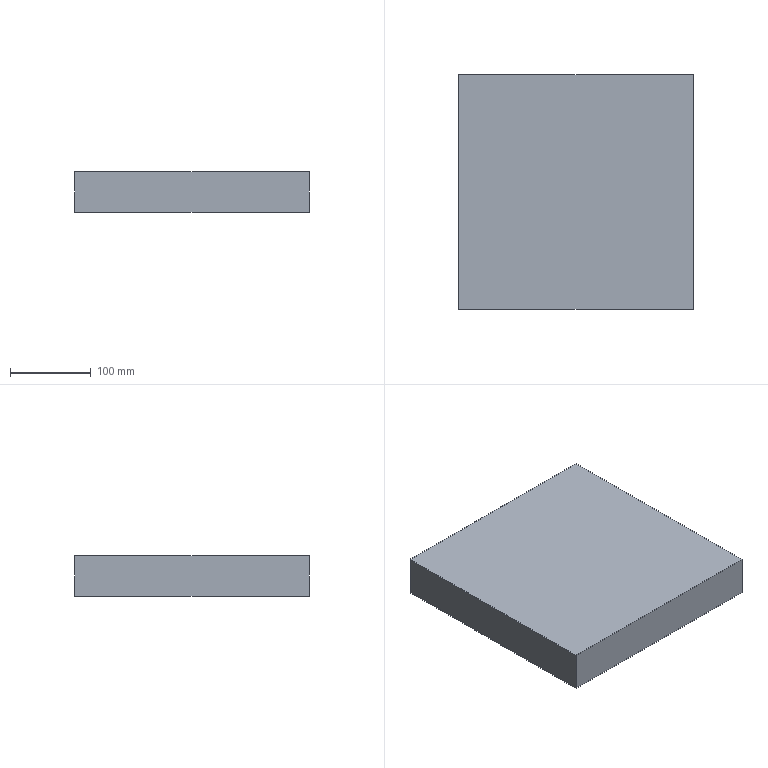Part | STEP file | SceondUPS_Default | 1 solid | 6 faces | box 290 x 290 x 50 mm | volume 4205000 mm3 | plane 6
STEP:
#1=CARTESIAN_POINT('',(0.,0.,0.));
#2=DIRECTION('',(0.,0.,1.));
#3=DIRECTION('',(1.,0.,0.));
#4=AXIS2_PLACEMENT_3D('',#1,#2,#3);
#5=CARTESIAN_POINT('',(0.,0.,-50.));
#6=VERTEX_POINT('',#5);
#7=CARTESIAN_POINT('',(0.,0.,0.));
#8=VERTEX_POINT('',#7);
#9=CARTESIAN_POINT('',(0.,0.,0.));
#10=DIRECTION('',(0.,0.,1.));
#11=VECTOR('',#10,1.);
#12=LINE('',#9,#11);
#13=CARTESIAN_POINT('',(0.,290.,0.));
#14=DIRECTION('',(1.,0.,0.));
#15=DIRECTION('',(0.,0.,-1.));
#16=AXIS2_PLACEMENT_3D('',#13,#14,#15);
#17=PLANE('',#16);
#18=CARTESIAN_POINT('',(0.,-290.));
#19=DIRECTION('',(-1.,0.));
#20=VECTOR('',#19,1.);
#21=LINE('',#18,#20);
#22=(GEOMETRIC_REPRESENTATION_CONTEXT(2)PARAMETRIC_REPRESENTATION_CONTEXT()REPRESENTATION_CONTEXT('',''));
#23=DEFINITIONAL_REPRESENTATION('',(#21),#22);
#24=PCURVE('',#17,#23);
#25=CARTESIAN_POINT('',(0.,0.,-50.));
#26=DIRECTION('',(0.,-1.,0.));
#27=DIRECTION('',(0.,0.,-1.));
#28=AXIS2_PLACEMENT_3D('',#25,#26,#27);
#29=PLANE('',#28);
#30=CARTESIAN_POINT('',(-50.,0.));
#31=DIRECTION('',(-1.,0.));
#32=VECTOR('',#31,1.);
#33=LINE('',#30,#32);
#34=(GEOMETRIC_REPRESENTATION_CONTEXT(2)PARAMETRIC_REPRESENTATION_CONTEXT()REPRESENTATION_CONTEXT('',''));
#35=DEFINITIONAL_REPRESENTATION('',(#33),#34);
#36=PCURVE('',#29,#35);
#37=SURFACE_CURVE('',#12,(#24,#36),.PCURVE_S1.);
#38=EDGE_CURVE('',#6,#8,#37,.T.);
#39=ORIENTED_EDGE('',*,*,#38,.T.);
#40=CARTESIAN_POINT('',(0.,290.,0.));
#41=VERTEX_POINT('',#40);
#42=CARTESIAN_POINT('',(0.,290.,0.));
#43=DIRECTION('',(0.,-1.,0.));
#44=VECTOR('',#43,1.);
#45=LINE('',#42,#44);
#46=CARTESIAN_POINT('',(0.,0.));
#47=DIRECTION('',(0.,-1.));
#48=VECTOR('',#47,1.);
#49=LINE('',#46,#48);
#50=(GEOMETRIC_REPRESENTATION_CONTEXT(2)PARAMETRIC_REPRESENTATION_CONTEXT()REPRESENTATION_CONTEXT('',''));
#51=DEFINITIONAL_REPRESENTATION('',(#49),#50);
#52=PCURVE('',#17,#51);
#53=CARTESIAN_POINT('',(0.,290.,0.));
#54=DIRECTION('',(0.,0.,-1.));
#55=DIRECTION('',(-1.,0.,0.));
#56=AXIS2_PLACEMENT_3D('',#53,#54,#55);
#57=PLANE('',#56);
#58=CARTESIAN_POINT('',(0.,0.));
#59=DIRECTION('',(0.,-1.));
#60=VECTOR('',#59,1.);
#61=LINE('',#58,#60);
#62=(GEOMETRIC_REPRESENTATION_CONTEXT(2)PARAMETRIC_REPRESENTATION_CONTEXT()REPRESENTATION_CONTEXT('',''));
#63=DEFINITIONAL_REPRESENTATION('',(#61),#62);
#64=PCURVE('',#57,#63);
#65=SURFACE_CURVE('',#45,(#52,#64),.PCURVE_S1.);
#66=EDGE_CURVE('',#41,#8,#65,.T.);
#67=ORIENTED_EDGE('',*,*,#66,.F.);
#68=CARTESIAN_POINT('',(0.,290.,-50.));
#69=VERTEX_POINT('',#68);
#70=CARTESIAN_POINT('',(0.,290.,0.));
#71=DIRECTION('',(0.,0.,1.));
#72=VECTOR('',#71,1.);
#73=LINE('',#70,#72);
#74=CARTESIAN_POINT('',(0.,0.));
#75=DIRECTION('',(-1.,0.));
#76=VECTOR('',#75,1.);
#77=LINE('',#74,#76);
#78=(GEOMETRIC_REPRESENTATION_CONTEXT(2)PARAMETRIC_REPRESENTATION_CONTEXT()REPRESENTATION_CONTEXT('',''));
#79=DEFINITIONAL_REPRESENTATION('',(#77),#78);
#80=PCURVE('',#17,#79);
#81=CARTESIAN_POINT('',(0.,290.,-50.));
#82=DIRECTION('',(0.,-1.,0.));
#83=DIRECTION('',(0.,0.,-1.));
#84=AXIS2_PLACEMENT_3D('',#81,#82,#83);
#85=PLANE('',#84);
#86=CARTESIAN_POINT('',(-50.,0.));
#87=DIRECTION('',(-1.,0.));
#88=VECTOR('',#87,1.);
#89=LINE('',#86,#88);
#90=(GEOMETRIC_REPRESENTATION_CONTEXT(2)PARAMETRIC_REPRESENTATION_CONTEXT()REPRESENTATION_CONTEXT('',''));
#91=DEFINITIONAL_REPRESENTATION('',(#89),#90);
#92=PCURVE('',#85,#91);
#93=SURFACE_CURVE('',#73,(#80,#92),.PCURVE_S1.);
#94=EDGE_CURVE('',#69,#41,#93,.T.);
#95=ORIENTED_EDGE('',*,*,#94,.F.);
#96=CARTESIAN_POINT('',(0.,290.,-50.));
#97=DIRECTION('',(0.,-1.,0.));
#98=VECTOR('',#97,1.);
#99=LINE('',#96,#98);
#100=CARTESIAN_POINT('',(50.,0.));
#101=DIRECTION('',(0.,-1.));
#102=VECTOR('',#101,1.);
#103=LINE('',#100,#102);
#104=(GEOMETRIC_REPRESENTATION_CONTEXT(2)PARAMETRIC_REPRESENTATION_CONTEXT()REPRESENTATION_CONTEXT('',''));
#105=DEFINITIONAL_REPRESENTATION('',(#103),#104);
#106=PCURVE('',#17,#105);
#107=CARTESIAN_POINT('',(0.,290.,-50.));
#108=DIRECTION('',(0.,0.,1.));
#109=DIRECTION('',(1.,0.,0.));
#110=AXIS2_PLACEMENT_3D('',#107,#108,#109);
#111=PLANE('',#110);
#112=CARTESIAN_POINT('',(0.,0.));
#113=DIRECTION('',(0.,-1.));
#114=VECTOR('',#113,1.);
#115=LINE('',#112,#114);
#116=(GEOMETRIC_REPRESENTATION_CONTEXT(2)PARAMETRIC_REPRESENTATION_CONTEXT()REPRESENTATION_CONTEXT('',''));
#117=DEFINITIONAL_REPRESENTATION('',(#115),#116);
#118=PCURVE('',#111,#117);
#119=SURFACE_CURVE('',#99,(#106,#118),.PCURVE_S1.);
#120=EDGE_CURVE('',#69,#6,#119,.T.);
#121=ORIENTED_EDGE('',*,*,#120,.T.);
#122=EDGE_LOOP('',(#39,#67,#95,#121));
#123=FACE_BOUND('',#122,.T.);
#124=ADVANCED_FACE('',(#123),#17,.F.);
#125=CARTESIAN_POINT('',(290.,0.,0.));
#126=VERTEX_POINT('',#125);
#127=CARTESIAN_POINT('',(0.,0.,0.));
#128=DIRECTION('',(1.,0.,0.));
#129=VECTOR('',#128,1.);
#130=LINE('',#127,#129);
#131=CARTESIAN_POINT('',(0.,-290.));
#132=DIRECTION('',(-1.,0.));
#133=VECTOR('',#132,1.);
#134=LINE('',#131,#133);
#135=(GEOMETRIC_REPRESENTATION_CONTEXT(2)PARAMETRIC_REPRESENTATION_CONTEXT()REPRESENTATION_CONTEXT('',''));
#136=DEFINITIONAL_REPRESENTATION('',(#134),#135);
#137=PCURVE('',#57,#136);
#138=CARTESIAN_POINT('',(-50.,0.));
#139=DIRECTION('',(0.,1.));
#140=VECTOR('',#139,1.);
#141=LINE('',#138,#140);
#142=(GEOMETRIC_REPRESENTATION_CONTEXT(2)PARAMETRIC_REPRESENTATION_CONTEXT()REPRESENTATION_CONTEXT('',''));
#143=DEFINITIONAL_REPRESENTATION('',(#141),#142);
#144=PCURVE('',#29,#143);
#145=SURFACE_CURVE('',#130,(#137,#144),.PCURVE_S1.);
#146=EDGE_CURVE('',#8,#126,#145,.T.);
#147=ORIENTED_EDGE('',*,*,#146,.T.);
#148=CARTESIAN_POINT('',(290.,290.,0.));
#149=VERTEX_POINT('',#148);
#150=CARTESIAN_POINT('',(290.,290.,0.));
#151=DIRECTION('',(0.,-1.,0.));
#152=VECTOR('',#151,1.);
#153=LINE('',#150,#152);
#154=CARTESIAN_POINT('',(-290.,0.));
#155=DIRECTION('',(0.,-1.));
#156=VECTOR('',#155,1.);
#157=LINE('',#154,#156);
#158=(GEOMETRIC_REPRESENTATION_CONTEXT(2)PARAMETRIC_REPRESENTATION_CONTEXT()REPRESENTATION_CONTEXT('',''));
#159=DEFINITIONAL_REPRESENTATION('',(#157),#158);
#160=PCURVE('',#57,#159);
#161=CARTESIAN_POINT('',(290.,290.,0.));
#162=DIRECTION('',(-1.,0.,0.));
#163=DIRECTION('',(0.,0.,1.));
#164=AXIS2_PLACEMENT_3D('',#161,#162,#163);
#165=PLANE('',#164);
#166=CARTESIAN_POINT('',(0.,0.));
#167=DIRECTION('',(0.,-1.));
#168=VECTOR('',#167,1.);
#169=LINE('',#166,#168);
#170=(GEOMETRIC_REPRESENTATION_CONTEXT(2)PARAMETRIC_REPRESENTATION_CONTEXT()REPRESENTATION_CONTEXT('',''));
#171=DEFINITIONAL_REPRESENTATION('',(#169),#170);
#172=PCURVE('',#165,#171);
#173=SURFACE_CURVE('',#153,(#160,#172),.PCURVE_S1.);
#174=EDGE_CURVE('',#149,#126,#173,.T.);
#175=ORIENTED_EDGE('',*,*,#174,.F.);
#176=CARTESIAN_POINT('',(0.,290.,0.));
#177=DIRECTION('',(1.,0.,0.));
#178=VECTOR('',#177,1.);
#179=LINE('',#176,#178);
#180=CARTESIAN_POINT('',(0.,0.));
#181=DIRECTION('',(-1.,0.));
#182=VECTOR('',#181,1.);
#183=LINE('',#180,#182);
#184=(GEOMETRIC_REPRESENTATION_CONTEXT(2)PARAMETRIC_REPRESENTATION_CONTEXT()REPRESENTATION_CONTEXT('',''));
#185=DEFINITIONAL_REPRESENTATION('',(#183),#184);
#186=PCURVE('',#57,#185);
#187=CARTESIAN_POINT('',(-50.,0.));
#188=DIRECTION('',(0.,1.));
#189=VECTOR('',#188,1.);
#190=LINE('',#187,#189);
#191=(GEOMETRIC_REPRESENTATION_CONTEXT(2)PARAMETRIC_REPRESENTATION_CONTEXT()REPRESENTATION_CONTEXT('',''));
#192=DEFINITIONAL_REPRESENTATION('',(#190),#191);
#193=PCURVE('',#85,#192);
#194=SURFACE_CURVE('',#179,(#186,#193),.PCURVE_S1.);
#195=EDGE_CURVE('',#41,#149,#194,.T.);
#196=ORIENTED_EDGE('',*,*,#195,.F.);
#197=ORIENTED_EDGE('',*,*,#66,.T.);
#198=EDGE_LOOP('',(#147,#175,#196,#197));
#199=FACE_BOUND('',#198,.T.);
#200=ADVANCED_FACE('',(#199),#57,.F.);
#201=CARTESIAN_POINT('',(290.,0.,-50.));
#202=VERTEX_POINT('',#201);
#203=CARTESIAN_POINT('',(290.,0.,0.));
#204=DIRECTION('',(0.,0.,-1.));
#205=VECTOR('',#204,1.);
#206=LINE('',#203,#205);
#207=CARTESIAN_POINT('',(0.,-290.));
#208=DIRECTION('',(-1.,0.));
#209=VECTOR('',#208,1.);
#210=LINE('',#207,#209);
#211=(GEOMETRIC_REPRESENTATION_CONTEXT(2)PARAMETRIC_REPRESENTATION_CONTEXT()REPRESENTATION_CONTEXT('',''));
#212=DEFINITIONAL_REPRESENTATION('',(#210),#211);
#213=PCURVE('',#165,#212);
#214=CARTESIAN_POINT('',(-50.,290.));
#215=DIRECTION('',(1.,0.));
#216=VECTOR('',#215,1.);
#217=LINE('',#214,#216);
#218=(GEOMETRIC_REPRESENTATION_CONTEXT(2)PARAMETRIC_REPRESENTATION_CONTEXT()REPRESENTATION_CONTEXT('',''));
#219=DEFINITIONAL_REPRESENTATION('',(#217),#218);
#220=PCURVE('',#29,#219);
#221=SURFACE_CURVE('',#206,(#213,#220),.PCURVE_S1.);
#222=EDGE_CURVE('',#126,#202,#221,.T.);
#223=ORIENTED_EDGE('',*,*,#222,.T.);
#224=CARTESIAN_POINT('',(290.,290.,-50.));
#225=VERTEX_POINT('',#224);
#226=CARTESIAN_POINT('',(290.,290.,-50.));
#227=DIRECTION('',(0.,-1.,0.));
#228=VECTOR('',#227,1.);
#229=LINE('',#226,#228);
#230=CARTESIAN_POINT('',(-50.,0.));
#231=DIRECTION('',(0.,-1.));
#232=VECTOR('',#231,1.);
#233=LINE('',#230,#232);
#234=(GEOMETRIC_REPRESENTATION_CONTEXT(2)PARAMETRIC_REPRESENTATION_CONTEXT()REPRESENTATION_CONTEXT('',''));
#235=DEFINITIONAL_REPRESENTATION('',(#233),#234);
#236=PCURVE('',#165,#235);
#237=CARTESIAN_POINT('',(290.,0.));
#238=DIRECTION('',(0.,-1.));
#239=VECTOR('',#238,1.);
#240=LINE('',#237,#239);
#241=(GEOMETRIC_REPRESENTATION_CONTEXT(2)PARAMETRIC_REPRESENTATION_CONTEXT()REPRESENTATION_CONTEXT('',''));
#242=DEFINITIONAL_REPRESENTATION('',(#240),#241);
#243=PCURVE('',#111,#242);
#244=SURFACE_CURVE('',#229,(#236,#243),.PCURVE_S1.);
#245=EDGE_CURVE('',#225,#202,#244,.T.);
#246=ORIENTED_EDGE('',*,*,#245,.F.);
#247=CARTESIAN_POINT('',(290.,290.,0.));
#248=DIRECTION('',(0.,0.,-1.));
#249=VECTOR('',#248,1.);
#250=LINE('',#247,#249);
#251=CARTESIAN_POINT('',(0.,0.));
#252=DIRECTION('',(-1.,0.));
#253=VECTOR('',#252,1.);
#254=LINE('',#251,#253);
#255=(GEOMETRIC_REPRESENTATION_CONTEXT(2)PARAMETRIC_REPRESENTATION_CONTEXT()REPRESENTATION_CONTEXT('',''));
#256=DEFINITIONAL_REPRESENTATION('',(#254),#255);
#257=PCURVE('',#165,#256);
#258=CARTESIAN_POINT('',(-50.,290.));
#259=DIRECTION('',(1.,0.));
#260=VECTOR('',#259,1.);
#261=LINE('',#258,#260);
#262=(GEOMETRIC_REPRESENTATION_CONTEXT(2)PARAMETRIC_REPRESENTATION_CONTEXT()REPRESENTATION_CONTEXT('',''));
#263=DEFINITIONAL_REPRESENTATION('',(#261),#262);
#264=PCURVE('',#85,#263);
#265=SURFACE_CURVE('',#250,(#257,#264),.PCURVE_S1.);
#266=EDGE_CURVE('',#149,#225,#265,.T.);
#267=ORIENTED_EDGE('',*,*,#266,.F.);
#268=ORIENTED_EDGE('',*,*,#174,.T.);
#269=EDGE_LOOP('',(#223,#246,#267,#268));
#270=FACE_BOUND('',#269,.T.);
#271=ADVANCED_FACE('',(#270),#165,.F.);
#272=CARTESIAN_POINT('',(0.,0.,-50.));
#273=DIRECTION('',(-1.,0.,0.));
#274=VECTOR('',#273,1.);
#275=LINE('',#272,#274);
#276=CARTESIAN_POINT('',(0.,-290.));
#277=DIRECTION('',(-1.,0.));
#278=VECTOR('',#277,1.);
#279=LINE('',#276,#278);
#280=(GEOMETRIC_REPRESENTATION_CONTEXT(2)PARAMETRIC_REPRESENTATION_CONTEXT()REPRESENTATION_CONTEXT('',''));
#281=DEFINITIONAL_REPRESENTATION('',(#279),#280);
#282=PCURVE('',#111,#281);
#283=CARTESIAN_POINT('',(0.,0.));
#284=DIRECTION('',(0.,-1.));
#285=VECTOR('',#284,1.);
#286=LINE('',#283,#285);
#287=(GEOMETRIC_REPRESENTATION_CONTEXT(2)PARAMETRIC_REPRESENTATION_CONTEXT()REPRESENTATION_CONTEXT('',''));
#288=DEFINITIONAL_REPRESENTATION('',(#286),#287);
#289=PCURVE('',#29,#288);
#290=SURFACE_CURVE('',#275,(#282,#289),.PCURVE_S1.);
#291=EDGE_CURVE('',#202,#6,#290,.T.);
#292=ORIENTED_EDGE('',*,*,#291,.T.);
#293=ORIENTED_EDGE('',*,*,#120,.F.);
#294=CARTESIAN_POINT('',(0.,290.,-50.));
#295=DIRECTION('',(-1.,0.,0.));
#296=VECTOR('',#295,1.);
#297=LINE('',#294,#296);
#298=CARTESIAN_POINT('',(0.,0.));
#299=DIRECTION('',(-1.,0.));
#300=VECTOR('',#299,1.);
#301=LINE('',#298,#300);
#302=(GEOMETRIC_REPRESENTATION_CONTEXT(2)PARAMETRIC_REPRESENTATION_CONTEXT()REPRESENTATION_CONTEXT('',''));
#303=DEFINITIONAL_REPRESENTATION('',(#301),#302);
#304=PCURVE('',#111,#303);
#305=CARTESIAN_POINT('',(0.,0.));
#306=DIRECTION('',(0.,-1.));
#307=VECTOR('',#306,1.);
#308=LINE('',#305,#307);
#309=(GEOMETRIC_REPRESENTATION_CONTEXT(2)PARAMETRIC_REPRESENTATION_CONTEXT()REPRESENTATION_CONTEXT('',''));
#310=DEFINITIONAL_REPRESENTATION('',(#308),#309);
#311=PCURVE('',#85,#310);
#312=SURFACE_CURVE('',#297,(#304,#311),.PCURVE_S1.);
#313=EDGE_CURVE('',#225,#69,#312,.T.);
#314=ORIENTED_EDGE('',*,*,#313,.F.);
#315=ORIENTED_EDGE('',*,*,#245,.T.);
#316=EDGE_LOOP('',(#292,#293,#314,#315));
#317=FACE_BOUND('',#316,.T.);
#318=ADVANCED_FACE('',(#317),#111,.F.);
#319=ORIENTED_EDGE('',*,*,#94,.T.);
#320=ORIENTED_EDGE('',*,*,#195,.T.);
#321=ORIENTED_EDGE('',*,*,#266,.T.);
#322=ORIENTED_EDGE('',*,*,#313,.T.);
#323=EDGE_LOOP('',(#319,#320,#321,#322));
#324=FACE_BOUND('',#323,.T.);
#325=ADVANCED_FACE('',(#324),#85,.F.);
#326=ORIENTED_EDGE('',*,*,#38,.F.);
#327=ORIENTED_EDGE('',*,*,#291,.F.);
#328=ORIENTED_EDGE('',*,*,#222,.F.);
#329=ORIENTED_EDGE('',*,*,#146,.F.);
#330=EDGE_LOOP('',(#326,#327,#328,#329));
#331=FACE_BOUND('',#330,.T.);
#332=ADVANCED_FACE('',(#331),#29,.T.);
#333=CLOSED_SHELL('',(#124,#200,#271,#318,#325,#332));
#334=MANIFOLD_SOLID_BREP('',#333);
#335=(LENGTH_UNIT()NAMED_UNIT(*)SI_UNIT(.MILLI.,.METRE.));
#336=UNCERTAINTY_MEASURE_WITH_UNIT(LENGTH_MEASURE(0.0000001),#335,'','');
#337=(NAMED_UNIT(*)PLANE_ANGLE_UNIT()SI_UNIT($,.RADIAN.));
#338=(NAMED_UNIT(*)SI_UNIT($,.STERADIAN.)SOLID_ANGLE_UNIT());
#339=(GEOMETRIC_REPRESENTATION_CONTEXT(3)GLOBAL_UNCERTAINTY_ASSIGNED_CONTEXT((#336))GLOBAL_UNIT_ASSIGNED_CONTEXT((#335,#337,#338))REPRESENTATION_CONTEXT('',''));
#340=ADVANCED_BREP_SHAPE_REPRESENTATION('',(#4,#334),#339);